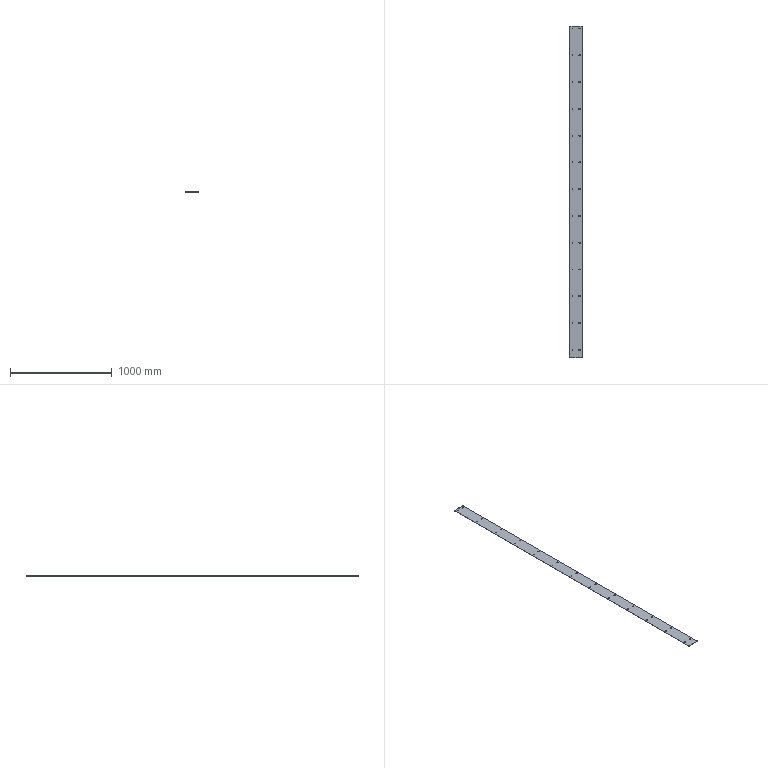Part | STEP file | Assembly TS-S03 | 1 solid | 103 faces | box 120 x 3256 x 2 mm | volume 777120 mm3 | cylinder 70 | plane 33 | commonest cylinder face diameters 8 x65 20 x4 10 x1